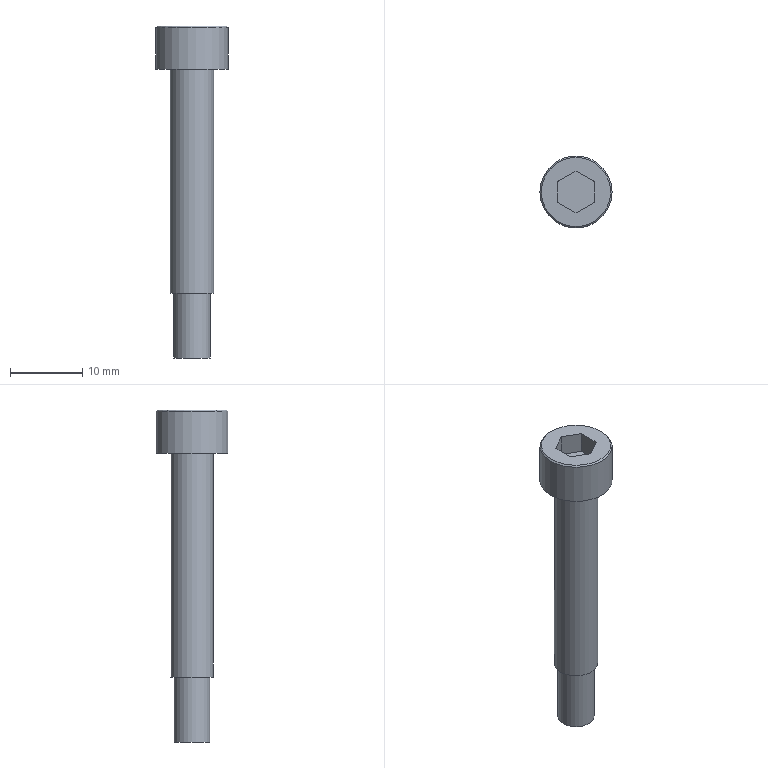Part | STEP file | M3-10_id274_x_t | 1 solid | 15 faces | box 10 x 10 x 46 mm | volume 1459 mm3 | plane 11 | cylinder 3 | cone 1 | commonest cylinder face diameters 5 x1 6 x1 10 x1
STEP:
#1=CARTESIAN_POINT('',(-204.,-85.,-47.));
#2=VERTEX_POINT('',#1);
#3=CARTESIAN_POINT('',(-201.5,-85.,-47.));
#4=DIRECTION('',(0.,0.,-1.));
#5=DIRECTION('',(-1.,0.,0.));
#6=AXIS2_PLACEMENT_3D('',#3,#4,#5);
#7=CIRCLE('',#6,2.5);
#8=EDGE_CURVE('',#2,#2,#7,.T.);
#9=ORIENTED_EDGE('',*,*,#8,.F.);
#10=EDGE_LOOP('',(#9));
#11=FACE_BOUND('',#10,.T.);
#12=CARTESIAN_POINT('',(-198.5,-85.,-47.));
#13=VERTEX_POINT('',#12);
#14=CARTESIAN_POINT('',(-201.5,-85.,-47.));
#15=DIRECTION('',(0.,0.,1.));
#16=DIRECTION('',(1.,0.,0.));
#17=AXIS2_PLACEMENT_3D('',#14,#15,#16);
#18=CIRCLE('',#17,3.);
#19=EDGE_CURVE('',#13,#13,#18,.T.);
#20=ORIENTED_EDGE('',*,*,#19,.F.);
#21=EDGE_LOOP('',(#20));
#22=FACE_BOUND('',#21,.T.);
#23=CARTESIAN_POINT('',(-201.5,-85.,-47.));
#24=DIRECTION('',(0.,0.,-1.));
#25=DIRECTION('',(-1.,0.,0.));
#26=AXIS2_PLACEMENT_3D('',#23,#24,#25);
#27=PLANE('',#26);
#28=ADVANCED_FACE('',(#11,#22),#27,.T.);
#29=CARTESIAN_POINT('',(-204.5,-85.,-16.));
#30=VERTEX_POINT('',#29);
#31=CARTESIAN_POINT('',(-201.5,-85.,-16.));
#32=DIRECTION('',(0.,0.,1.));
#33=DIRECTION('',(-1.,0.,0.));
#34=AXIS2_PLACEMENT_3D('',#31,#32,#33);
#35=CIRCLE('',#34,3.);
#36=EDGE_CURVE('',#30,#30,#35,.T.);
#37=ORIENTED_EDGE('',*,*,#36,.F.);
#38=EDGE_LOOP('',(#37));
#39=FACE_BOUND('',#38,.T.);
#40=ORIENTED_EDGE('',*,*,#19,.T.);
#41=EDGE_LOOP('',(#40));
#42=FACE_BOUND('',#41,.T.);
#43=CARTESIAN_POINT('',(-201.5,-85.,-47.));
#44=DIRECTION('',(0.,0.,1.));
#45=DIRECTION('',(1.,0.,0.));
#46=AXIS2_PLACEMENT_3D('',#43,#44,#45);
#47=CYLINDRICAL_SURFACE('',#46,3.);
#48=ADVANCED_FACE('',(#39,#42),#47,.T.);
#49=CARTESIAN_POINT('',(-199.,-85.,-56.));
#50=VERTEX_POINT('',#49);
#51=CARTESIAN_POINT('',(-201.5,-85.,-56.));
#52=DIRECTION('',(0.,0.,1.));
#53=DIRECTION('',(1.,0.,0.));
#54=AXIS2_PLACEMENT_3D('',#51,#52,#53);
#55=CIRCLE('',#54,2.5);
#56=EDGE_CURVE('',#50,#50,#55,.T.);
#57=ORIENTED_EDGE('',*,*,#56,.F.);
#58=EDGE_LOOP('',(#57));
#59=FACE_OUTER_BOUND('',#58,.T.);
#60=CARTESIAN_POINT('',(-201.5,-85.,-56.));
#61=DIRECTION('',(0.,0.,-1.));
#62=DIRECTION('',(-1.,0.,0.));
#63=AXIS2_PLACEMENT_3D('',#60,#61,#62);
#64=PLANE('',#63);
#65=ADVANCED_FACE('',(#59),#64,.T.);
#66=ORIENTED_EDGE('',*,*,#56,.T.);
#67=EDGE_LOOP('',(#66));
#68=FACE_BOUND('',#67,.T.);
#69=ORIENTED_EDGE('',*,*,#8,.T.);
#70=EDGE_LOOP('',(#69));
#71=FACE_BOUND('',#70,.T.);
#72=CARTESIAN_POINT('',(-201.5,-85.,-47.));
#73=DIRECTION('',(0.,0.,-1.));
#74=DIRECTION('',(1.,0.,0.));
#75=AXIS2_PLACEMENT_3D('',#72,#73,#74);
#76=CYLINDRICAL_SURFACE('',#75,2.5);
#77=ADVANCED_FACE('',(#68,#71),#76,.T.);
#78=CARTESIAN_POINT('',(-204.,-83.557,-10.));
#79=VERTEX_POINT('',#78);
#80=CARTESIAN_POINT('',(-204.,-86.443,-10.));
#81=VERTEX_POINT('',#80);
#82=CARTESIAN_POINT('',(-204.,-83.557,-10.));
#83=DIRECTION('',(0.,-1.,0.));
#84=VECTOR('',#83,1.);
#85=LINE('',#82,#84);
#86=EDGE_CURVE('',#79,#81,#85,.T.);
#87=ORIENTED_EDGE('',*,*,#86,.F.);
#88=CARTESIAN_POINT('',(-201.5,-82.113,-10.));
#89=VERTEX_POINT('',#88);
#90=CARTESIAN_POINT('',(-201.5,-82.113,-10.));
#91=DIRECTION('',(-0.866,-0.5,0.));
#92=VECTOR('',#91,1.);
#93=LINE('',#90,#92);
#94=EDGE_CURVE('',#89,#79,#93,.T.);
#95=ORIENTED_EDGE('',*,*,#94,.F.);
#96=CARTESIAN_POINT('',(-199.,-83.557,-10.));
#97=VERTEX_POINT('',#96);
#98=CARTESIAN_POINT('',(-199.,-83.557,-10.));
#99=DIRECTION('',(-0.866,0.5,0.));
#100=VECTOR('',#99,1.);
#101=LINE('',#98,#100);
#102=EDGE_CURVE('',#97,#89,#101,.T.);
#103=ORIENTED_EDGE('',*,*,#102,.F.);
#104=CARTESIAN_POINT('',(-199.,-86.443,-10.));
#105=VERTEX_POINT('',#104);
#106=CARTESIAN_POINT('',(-199.,-86.443,-10.));
#107=DIRECTION('',(0.,1.,0.));
#108=VECTOR('',#107,1.);
#109=LINE('',#106,#108);
#110=EDGE_CURVE('',#105,#97,#109,.T.);
#111=ORIENTED_EDGE('',*,*,#110,.F.);
#112=CARTESIAN_POINT('',(-201.5,-87.887,-10.));
#113=VERTEX_POINT('',#112);
#114=CARTESIAN_POINT('',(-201.5,-87.887,-10.));
#115=DIRECTION('',(0.866,0.5,0.));
#116=VECTOR('',#115,1.);
#117=LINE('',#114,#116);
#118=EDGE_CURVE('',#113,#105,#117,.T.);
#119=ORIENTED_EDGE('',*,*,#118,.F.);
#120=CARTESIAN_POINT('',(-204.,-86.443,-10.));
#121=DIRECTION('',(0.866,-0.5,0.));
#122=VECTOR('',#121,1.);
#123=LINE('',#120,#122);
#124=EDGE_CURVE('',#81,#113,#123,.T.);
#125=ORIENTED_EDGE('',*,*,#124,.F.);
#126=EDGE_LOOP('',(#87,#95,#103,#111,#119,#125));
#127=FACE_BOUND('',#126,.T.);
#128=CARTESIAN_POINT('',(-196.7,-85.,-10.));
#129=VERTEX_POINT('',#128);
#130=CARTESIAN_POINT('',(-201.5,-85.,-10.));
#131=DIRECTION('',(0.,0.,1.));
#132=DIRECTION('',(1.,0.,0.));
#133=AXIS2_PLACEMENT_3D('',#130,#131,#132);
#134=CIRCLE('',#133,4.8);
#135=EDGE_CURVE('',#129,#129,#134,.T.);
#136=ORIENTED_EDGE('',*,*,#135,.T.);
#137=EDGE_LOOP('',(#136));
#138=FACE_BOUND('',#137,.T.);
#139=CARTESIAN_POINT('',(-201.5,-85.,-10.));
#140=DIRECTION('',(0.,0.,1.));
#141=DIRECTION('',(1.,0.,0.));
#142=AXIS2_PLACEMENT_3D('',#139,#140,#141);
#143=PLANE('',#142);
#144=ADVANCED_FACE('',(#127,#138),#143,.T.);
#145=ORIENTED_EDGE('',*,*,#36,.T.);
#146=EDGE_LOOP('',(#145));
#147=FACE_BOUND('',#146,.T.);
#148=CARTESIAN_POINT('',(-196.5,-85.,-16.));
#149=VERTEX_POINT('',#148);
#150=CARTESIAN_POINT('',(-201.5,-85.,-16.));
#151=DIRECTION('',(0.,0.,1.));
#152=DIRECTION('',(1.,0.,0.));
#153=AXIS2_PLACEMENT_3D('',#150,#151,#152);
#154=CIRCLE('',#153,5.);
#155=EDGE_CURVE('',#149,#149,#154,.T.);
#156=ORIENTED_EDGE('',*,*,#155,.F.);
#157=EDGE_LOOP('',(#156));
#158=FACE_BOUND('',#157,.T.);
#159=CARTESIAN_POINT('',(-201.5,-85.,-16.));
#160=DIRECTION('',(0.,0.,-1.));
#161=DIRECTION('',(-1.,0.,0.));
#162=AXIS2_PLACEMENT_3D('',#159,#160,#161);
#163=PLANE('',#162);
#164=ADVANCED_FACE('',(#147,#158),#163,.T.);
#165=CARTESIAN_POINT('',(-196.5,-85.,-10.2));
#166=VERTEX_POINT('',#165);
#167=CARTESIAN_POINT('',(-201.5,-85.,-10.2));
#168=DIRECTION('',(0.,0.,-1.));
#169=DIRECTION('',(1.,0.,0.));
#170=AXIS2_PLACEMENT_3D('',#167,#168,#169);
#171=CIRCLE('',#170,5.);
#172=EDGE_CURVE('',#166,#166,#171,.T.);
#173=ORIENTED_EDGE('',*,*,#172,.T.);
#174=EDGE_LOOP('',(#173));
#175=FACE_BOUND('',#174,.T.);
#176=ORIENTED_EDGE('',*,*,#155,.T.);
#177=EDGE_LOOP('',(#176));
#178=FACE_BOUND('',#177,.T.);
#179=CARTESIAN_POINT('',(-201.5,-85.,-16.));
#180=DIRECTION('',(0.,0.,1.));
#181=DIRECTION('',(1.,0.,0.));
#182=AXIS2_PLACEMENT_3D('',#179,#180,#181);
#183=CYLINDRICAL_SURFACE('',#182,5.);
#184=ADVANCED_FACE('',(#175,#178),#183,.T.);
#185=ORIENTED_EDGE('',*,*,#135,.F.);
#186=EDGE_LOOP('',(#185));
#187=FACE_BOUND('',#186,.T.);
#188=ORIENTED_EDGE('',*,*,#172,.F.);
#189=EDGE_LOOP('',(#188));
#190=FACE_BOUND('',#189,.T.);
#191=CARTESIAN_POINT('',(-201.5,-85.,-10.2));
#192=DIRECTION('',(0.,0.,-1.));
#193=DIRECTION('',(-1.,0.,0.));
#194=AXIS2_PLACEMENT_3D('',#191,#192,#193);
#195=CONICAL_SURFACE('',#194,5.,45.);
#196=ADVANCED_FACE('',(#187,#190),#195,.T.);
#197=ORIENTED_EDGE('',*,*,#86,.T.);
#198=CARTESIAN_POINT('',(-204.,-86.443,-13.));
#199=VERTEX_POINT('',#198);
#200=CARTESIAN_POINT('',(-204.,-86.443,-13.));
#201=DIRECTION('',(0.,0.,-1.));
#202=VECTOR('',#201,1.);
#203=LINE('',#200,#202);
#204=EDGE_CURVE('',#81,#199,#203,.T.);
#205=ORIENTED_EDGE('',*,*,#204,.T.);
#206=CARTESIAN_POINT('',(-204.,-83.557,-13.));
#207=VERTEX_POINT('',#206);
#208=CARTESIAN_POINT('',(-204.,-83.557,-13.));
#209=DIRECTION('',(0.,1.,0.));
#210=VECTOR('',#209,1.);
#211=LINE('',#208,#210);
#212=EDGE_CURVE('',#199,#207,#211,.T.);
#213=ORIENTED_EDGE('',*,*,#212,.T.);
#214=CARTESIAN_POINT('',(-204.,-83.557,-13.));
#215=DIRECTION('',(0.,0.,-1.));
#216=VECTOR('',#215,1.);
#217=LINE('',#214,#216);
#218=EDGE_CURVE('',#79,#207,#217,.T.);
#219=ORIENTED_EDGE('',*,*,#218,.F.);
#220=EDGE_LOOP('',(#197,#205,#213,#219));
#221=FACE_OUTER_BOUND('',#220,.T.);
#222=CARTESIAN_POINT('',(-204.,-83.557,-13.));
#223=DIRECTION('',(-1.,0.,0.));
#224=DIRECTION('',(0.,-1.,0.));
#225=AXIS2_PLACEMENT_3D('',#222,#223,#224);
#226=PLANE('',#225);
#227=ADVANCED_FACE('',(#221),#226,.F.);
#228=ORIENTED_EDGE('',*,*,#124,.T.);
#229=CARTESIAN_POINT('',(-201.5,-87.887,-13.));
#230=VERTEX_POINT('',#229);
#231=CARTESIAN_POINT('',(-201.5,-87.887,-13.));
#232=DIRECTION('',(0.,0.,-1.));
#233=VECTOR('',#232,1.);
#234=LINE('',#231,#233);
#235=EDGE_CURVE('',#113,#230,#234,.T.);
#236=ORIENTED_EDGE('',*,*,#235,.T.);
#237=CARTESIAN_POINT('',(-204.,-86.443,-13.));
#238=DIRECTION('',(-0.866,0.5,0.));
#239=VECTOR('',#238,1.);
#240=LINE('',#237,#239);
#241=EDGE_CURVE('',#230,#199,#240,.T.);
#242=ORIENTED_EDGE('',*,*,#241,.T.);
#243=ORIENTED_EDGE('',*,*,#204,.F.);
#244=EDGE_LOOP('',(#228,#236,#242,#243));
#245=FACE_OUTER_BOUND('',#244,.T.);
#246=CARTESIAN_POINT('',(-204.,-86.443,-13.));
#247=DIRECTION('',(-0.5,-0.866,0.));
#248=DIRECTION('',(0.866,-0.5,0.));
#249=AXIS2_PLACEMENT_3D('',#246,#247,#248);
#250=PLANE('',#249);
#251=ADVANCED_FACE('',(#245),#250,.F.);
#252=ORIENTED_EDGE('',*,*,#118,.T.);
#253=CARTESIAN_POINT('',(-199.,-86.443,-13.));
#254=VERTEX_POINT('',#253);
#255=CARTESIAN_POINT('',(-199.,-86.443,-13.));
#256=DIRECTION('',(0.,0.,-1.));
#257=VECTOR('',#256,1.);
#258=LINE('',#255,#257);
#259=EDGE_CURVE('',#105,#254,#258,.T.);
#260=ORIENTED_EDGE('',*,*,#259,.T.);
#261=CARTESIAN_POINT('',(-201.5,-87.887,-13.));
#262=DIRECTION('',(-0.866,-0.5,0.));
#263=VECTOR('',#262,1.);
#264=LINE('',#261,#263);
#265=EDGE_CURVE('',#254,#230,#264,.T.);
#266=ORIENTED_EDGE('',*,*,#265,.T.);
#267=ORIENTED_EDGE('',*,*,#235,.F.);
#268=EDGE_LOOP('',(#252,#260,#266,#267));
#269=FACE_OUTER_BOUND('',#268,.T.);
#270=CARTESIAN_POINT('',(-201.5,-87.887,-13.));
#271=DIRECTION('',(0.5,-0.866,0.));
#272=DIRECTION('',(0.866,0.5,0.));
#273=AXIS2_PLACEMENT_3D('',#270,#271,#272);
#274=PLANE('',#273);
#275=ADVANCED_FACE('',(#269),#274,.F.);
#276=ORIENTED_EDGE('',*,*,#110,.T.);
#277=CARTESIAN_POINT('',(-199.,-83.557,-13.));
#278=VERTEX_POINT('',#277);
#279=CARTESIAN_POINT('',(-199.,-83.557,-13.));
#280=DIRECTION('',(0.,0.,-1.));
#281=VECTOR('',#280,1.);
#282=LINE('',#279,#281);
#283=EDGE_CURVE('',#97,#278,#282,.T.);
#284=ORIENTED_EDGE('',*,*,#283,.T.);
#285=CARTESIAN_POINT('',(-199.,-86.443,-13.));
#286=DIRECTION('',(0.,-1.,0.));
#287=VECTOR('',#286,1.);
#288=LINE('',#285,#287);
#289=EDGE_CURVE('',#278,#254,#288,.T.);
#290=ORIENTED_EDGE('',*,*,#289,.T.);
#291=ORIENTED_EDGE('',*,*,#259,.F.);
#292=EDGE_LOOP('',(#276,#284,#290,#291));
#293=FACE_OUTER_BOUND('',#292,.T.);
#294=CARTESIAN_POINT('',(-199.,-86.443,-13.));
#295=DIRECTION('',(1.,0.,0.));
#296=DIRECTION('',(0.,1.,0.));
#297=AXIS2_PLACEMENT_3D('',#294,#295,#296);
#298=PLANE('',#297);
#299=ADVANCED_FACE('',(#293),#298,.F.);
#300=ORIENTED_EDGE('',*,*,#102,.T.);
#301=CARTESIAN_POINT('',(-201.5,-82.113,-13.));
#302=VERTEX_POINT('',#301);
#303=CARTESIAN_POINT('',(-201.5,-82.113,-13.));
#304=DIRECTION('',(0.,0.,-1.));
#305=VECTOR('',#304,1.);
#306=LINE('',#303,#305);
#307=EDGE_CURVE('',#89,#302,#306,.T.);
#308=ORIENTED_EDGE('',*,*,#307,.T.);
#309=CARTESIAN_POINT('',(-199.,-83.557,-13.));
#310=DIRECTION('',(0.866,-0.5,0.));
#311=VECTOR('',#310,1.);
#312=LINE('',#309,#311);
#313=EDGE_CURVE('',#302,#278,#312,.T.);
#314=ORIENTED_EDGE('',*,*,#313,.T.);
#315=ORIENTED_EDGE('',*,*,#283,.F.);
#316=EDGE_LOOP('',(#300,#308,#314,#315));
#317=FACE_OUTER_BOUND('',#316,.T.);
#318=CARTESIAN_POINT('',(-199.,-83.557,-13.));
#319=DIRECTION('',(0.5,0.866,0.));
#320=DIRECTION('',(-0.866,0.5,0.));
#321=AXIS2_PLACEMENT_3D('',#318,#319,#320);
#322=PLANE('',#321);
#323=ADVANCED_FACE('',(#317),#322,.F.);
#324=ORIENTED_EDGE('',*,*,#94,.T.);
#325=ORIENTED_EDGE('',*,*,#218,.T.);
#326=CARTESIAN_POINT('',(-201.5,-82.113,-13.));
#327=DIRECTION('',(0.866,0.5,0.));
#328=VECTOR('',#327,1.);
#329=LINE('',#326,#328);
#330=EDGE_CURVE('',#207,#302,#329,.T.);
#331=ORIENTED_EDGE('',*,*,#330,.T.);
#332=ORIENTED_EDGE('',*,*,#307,.F.);
#333=EDGE_LOOP('',(#324,#325,#331,#332));
#334=FACE_OUTER_BOUND('',#333,.T.);
#335=CARTESIAN_POINT('',(-201.5,-82.113,-13.));
#336=DIRECTION('',(-0.5,0.866,0.));
#337=DIRECTION('',(-0.866,-0.5,0.));
#338=AXIS2_PLACEMENT_3D('',#335,#336,#337);
#339=PLANE('',#338);
#340=ADVANCED_FACE('',(#334),#339,.F.);
#341=ORIENTED_EDGE('',*,*,#212,.F.);
#342=ORIENTED_EDGE('',*,*,#241,.F.);
#343=ORIENTED_EDGE('',*,*,#265,.F.);
#344=ORIENTED_EDGE('',*,*,#289,.F.);
#345=ORIENTED_EDGE('',*,*,#313,.F.);
#346=ORIENTED_EDGE('',*,*,#330,.F.);
#347=EDGE_LOOP('',(#341,#342,#343,#344,#345,#346));
#348=FACE_OUTER_BOUND('',#347,.T.);
#349=CARTESIAN_POINT('',(-201.5,-85.,-13.));
#350=DIRECTION('',(0.,0.,1.));
#351=DIRECTION('',(1.,0.,0.));
#352=AXIS2_PLACEMENT_3D('',#349,#350,#351);
#353=PLANE('',#352);
#354=ADVANCED_FACE('',(#348),#353,.T.);
#355=CLOSED_SHELL('',(#28,#48,#65,#77,#144,#164,#184,#196,#227,#251,#275,#299,#323,#340,#354));
#356=MANIFOLD_SOLID_BREP('',#355);
#357=(LENGTH_UNIT()NAMED_UNIT(*)SI_UNIT(.MILLI.,.METRE.));
#358=UNCERTAINTY_MEASURE_WITH_UNIT(LENGTH_MEASURE(0.00002),#357,'','');
#359=(NAMED_UNIT(*)PLANE_ANGLE_UNIT()SI_UNIT($,.RADIAN.));
#360=PLANE_ANGLE_MEASURE_WITH_UNIT(PLANE_ANGLE_MEASURE(0.01745),#359);
#361=DIMENSIONAL_EXPONENTS(0.,0.,0.,0.,0.,0.,0.);
#362=(CONVERSION_BASED_UNIT('DEGREE',#360)NAMED_UNIT(#361)PLANE_ANGLE_UNIT());
#363=(NAMED_UNIT(*)SI_UNIT($,.STERADIAN.)SOLID_ANGLE_UNIT());
#364=(GEOMETRIC_REPRESENTATION_CONTEXT(3)GLOBAL_UNCERTAINTY_ASSIGNED_CONTEXT((#358))GLOBAL_UNIT_ASSIGNED_CONTEXT((#357,#362,#363))REPRESENTATION_CONTEXT('',''));
#365=ADVANCED_BREP_SHAPE_REPRESENTATION('',(#356),#364);